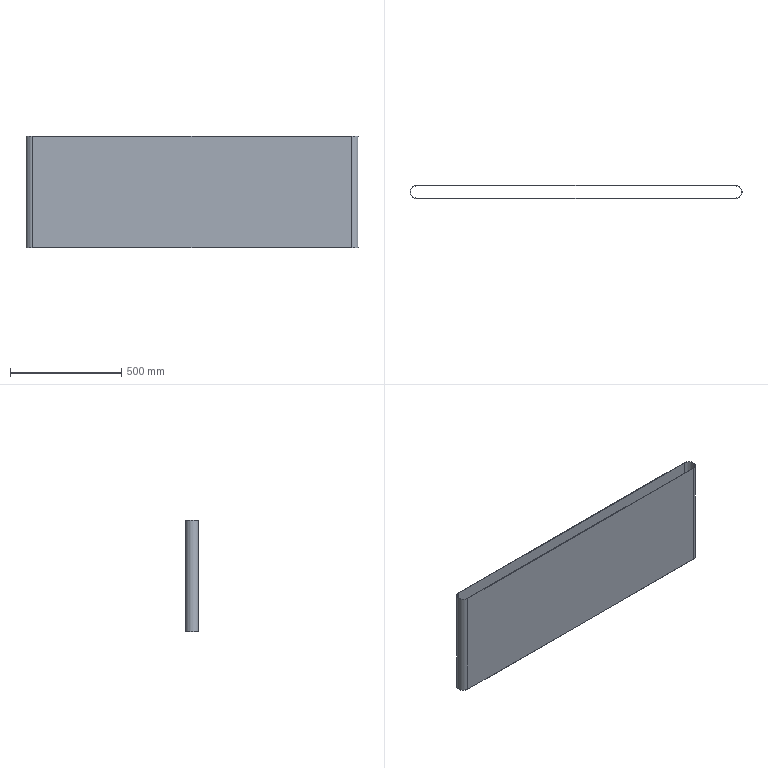Part | STEP file | RUBE Q7C | 1 solid | 10 faces | box 1492 x 59.6 x 500 mm | volume 2741026 mm3 | plane 6 | cylinder 4 | commonest cylinder face diameters 56 x2 59.6 x2
STEP:
#1=CARTESIAN_POINT('',(0.,0.,0.));
#2=DIRECTION('',(0.,0.,1.));
#3=DIRECTION('',(1.,0.,0.));
#4=AXIS2_PLACEMENT_3D('',#1,#2,#3);
#5=CARTESIAN_POINT('',(-1248.5,29.8,250.));
#6=VERTEX_POINT('',#5);
#7=CARTESIAN_POINT('',(-1248.5,-29.8,250.));
#8=VERTEX_POINT('',#7);
#9=CARTESIAN_POINT('',(-1248.5,0.,250.));
#10=DIRECTION('',(0.,0.,1.));
#11=DIRECTION('',(1.,0.,0.));
#12=AXIS2_PLACEMENT_3D('',#9,#10,#11);
#13=CIRCLE('',#12,29.8);
#14=CARTESIAN_POINT('',(-1248.5,0.,250.));
#15=DIRECTION('',(0.,0.,1.));
#16=DIRECTION('',(1.,0.,0.));
#17=AXIS2_PLACEMENT_3D('',#14,#15,#16);
#18=PLANE('',#17);
#19=CARTESIAN_POINT('',(0.,0.));
#20=DIRECTION('',(1.,0.));
#21=AXIS2_PLACEMENT_2D('',#19,#20);
#22=CIRCLE('',#21,29.8);
#23=(GEOMETRIC_REPRESENTATION_CONTEXT(2)PARAMETRIC_REPRESENTATION_CONTEXT()REPRESENTATION_CONTEXT('',''));
#24=DEFINITIONAL_REPRESENTATION('',(#22),#23);
#25=PCURVE('',#18,#24);
#26=CARTESIAN_POINT('',(-1248.5,0.,250.));
#27=DIRECTION('',(0.,0.,-1.));
#28=DIRECTION('',(-1.,0.,0.));
#29=AXIS2_PLACEMENT_3D('',#26,#27,#28);
#30=CYLINDRICAL_SURFACE('',#29,29.8);
#31=CARTESIAN_POINT('',(3.142,0.));
#32=DIRECTION('',(-1.,0.));
#33=VECTOR('',#32,1.);
#34=LINE('',#31,#33);
#35=(GEOMETRIC_REPRESENTATION_CONTEXT(2)PARAMETRIC_REPRESENTATION_CONTEXT()REPRESENTATION_CONTEXT('',''));
#36=DEFINITIONAL_REPRESENTATION('',(#34),#35);
#37=PCURVE('',#30,#36);
#38=SURFACE_CURVE('',#13,(#25,#37),.PCURVE_S1.);
#39=EDGE_CURVE('',#6,#8,#38,.T.);
#40=ORIENTED_EDGE('',*,*,#39,.T.);
#41=CARTESIAN_POINT('',(183.5,-29.8,250.));
#42=VERTEX_POINT('',#41);
#43=CARTESIAN_POINT('',(-1248.5,-29.8,250.));
#44=DIRECTION('',(1.,0.,0.));
#45=VECTOR('',#44,1.);
#46=LINE('',#43,#45);
#47=CARTESIAN_POINT('',(0.,-29.8));
#48=DIRECTION('',(1.,0.));
#49=VECTOR('',#48,1.);
#50=LINE('',#47,#49);
#51=(GEOMETRIC_REPRESENTATION_CONTEXT(2)PARAMETRIC_REPRESENTATION_CONTEXT()REPRESENTATION_CONTEXT('',''));
#52=DEFINITIONAL_REPRESENTATION('',(#50),#51);
#53=PCURVE('',#18,#52);
#54=CARTESIAN_POINT('',(-1248.5,-29.8,250.));
#55=DIRECTION('',(0.,1.,0.));
#56=DIRECTION('',(-1.,0.,0.));
#57=AXIS2_PLACEMENT_3D('',#54,#55,#56);
#58=PLANE('',#57);
#59=CARTESIAN_POINT('',(0.,0.));
#60=DIRECTION('',(-1.,0.));
#61=VECTOR('',#60,1.);
#62=LINE('',#59,#61);
#63=(GEOMETRIC_REPRESENTATION_CONTEXT(2)PARAMETRIC_REPRESENTATION_CONTEXT()REPRESENTATION_CONTEXT('',''));
#64=DEFINITIONAL_REPRESENTATION('',(#62),#63);
#65=PCURVE('',#58,#64);
#66=SURFACE_CURVE('',#46,(#53,#65),.PCURVE_S1.);
#67=EDGE_CURVE('',#8,#42,#66,.T.);
#68=ORIENTED_EDGE('',*,*,#67,.T.);
#69=CARTESIAN_POINT('',(183.5,29.8,250.));
#70=VERTEX_POINT('',#69);
#71=CARTESIAN_POINT('',(183.5,0.,250.));
#72=DIRECTION('',(0.,0.,1.));
#73=DIRECTION('',(1.,0.,0.));
#74=AXIS2_PLACEMENT_3D('',#71,#72,#73);
#75=CIRCLE('',#74,29.8);
#76=CARTESIAN_POINT('',(1432.,0.));
#77=DIRECTION('',(1.,0.));
#78=AXIS2_PLACEMENT_2D('',#76,#77);
#79=CIRCLE('',#78,29.8);
#80=(GEOMETRIC_REPRESENTATION_CONTEXT(2)PARAMETRIC_REPRESENTATION_CONTEXT()REPRESENTATION_CONTEXT('',''));
#81=DEFINITIONAL_REPRESENTATION('',(#79),#80);
#82=PCURVE('',#18,#81);
#83=CARTESIAN_POINT('',(183.5,0.,250.));
#84=DIRECTION('',(0.,0.,-1.));
#85=DIRECTION('',(-1.,0.,0.));
#86=AXIS2_PLACEMENT_3D('',#83,#84,#85);
#87=CYLINDRICAL_SURFACE('',#86,29.8);
#88=CARTESIAN_POINT('',(9.425,0.));
#89=DIRECTION('',(-1.,0.));
#90=VECTOR('',#89,1.);
#91=LINE('',#88,#90);
#92=(GEOMETRIC_REPRESENTATION_CONTEXT(2)PARAMETRIC_REPRESENTATION_CONTEXT()REPRESENTATION_CONTEXT('',''));
#93=DEFINITIONAL_REPRESENTATION('',(#91),#92);
#94=PCURVE('',#87,#93);
#95=SURFACE_CURVE('',#75,(#82,#94),.PCURVE_S1.);
#96=EDGE_CURVE('',#42,#70,#95,.T.);
#97=ORIENTED_EDGE('',*,*,#96,.T.);
#98=CARTESIAN_POINT('',(-1248.5,29.8,250.));
#99=DIRECTION('',(-1.,0.,0.));
#100=VECTOR('',#99,1.);
#101=LINE('',#98,#100);
#102=CARTESIAN_POINT('',(0.,29.8));
#103=DIRECTION('',(-1.,0.));
#104=VECTOR('',#103,1.);
#105=LINE('',#102,#104);
#106=(GEOMETRIC_REPRESENTATION_CONTEXT(2)PARAMETRIC_REPRESENTATION_CONTEXT()REPRESENTATION_CONTEXT('',''));
#107=DEFINITIONAL_REPRESENTATION('',(#105),#106);
#108=PCURVE('',#18,#107);
#109=CARTESIAN_POINT('',(-1248.5,29.8,250.));
#110=DIRECTION('',(0.,-1.,0.));
#111=DIRECTION('',(1.,0.,0.));
#112=AXIS2_PLACEMENT_3D('',#109,#110,#111);
#113=PLANE('',#112);
#114=CARTESIAN_POINT('',(0.,0.));
#115=DIRECTION('',(-1.,0.));
#116=VECTOR('',#115,1.);
#117=LINE('',#114,#116);
#118=(GEOMETRIC_REPRESENTATION_CONTEXT(2)PARAMETRIC_REPRESENTATION_CONTEXT()REPRESENTATION_CONTEXT('',''));
#119=DEFINITIONAL_REPRESENTATION('',(#117),#118);
#120=PCURVE('',#113,#119);
#121=SURFACE_CURVE('',#101,(#108,#120),.PCURVE_S1.);
#122=EDGE_CURVE('',#70,#6,#121,.T.);
#123=ORIENTED_EDGE('',*,*,#122,.T.);
#124=EDGE_LOOP('',(#40,#68,#97,#123));
#125=FACE_BOUND('',#124,.T.);
#126=CARTESIAN_POINT('',(-1248.5,-28.,250.));
#127=VERTEX_POINT('',#126);
#128=CARTESIAN_POINT('',(183.5,-28.,250.));
#129=VERTEX_POINT('',#128);
#130=CARTESIAN_POINT('',(-1248.5,-28.,250.));
#131=DIRECTION('',(1.,0.,0.));
#132=VECTOR('',#131,1.);
#133=LINE('',#130,#132);
#134=CARTESIAN_POINT('',(0.,-28.));
#135=DIRECTION('',(1.,0.));
#136=VECTOR('',#135,1.);
#137=LINE('',#134,#136);
#138=(GEOMETRIC_REPRESENTATION_CONTEXT(2)PARAMETRIC_REPRESENTATION_CONTEXT()REPRESENTATION_CONTEXT('',''));
#139=DEFINITIONAL_REPRESENTATION('',(#137),#138);
#140=PCURVE('',#18,#139);
#141=CARTESIAN_POINT('',(-1248.5,-28.,250.));
#142=DIRECTION('',(0.,1.,0.));
#143=DIRECTION('',(-1.,0.,0.));
#144=AXIS2_PLACEMENT_3D('',#141,#142,#143);
#145=PLANE('',#144);
#146=CARTESIAN_POINT('',(0.,0.));
#147=DIRECTION('',(-1.,0.));
#148=VECTOR('',#147,1.);
#149=LINE('',#146,#148);
#150=(GEOMETRIC_REPRESENTATION_CONTEXT(2)PARAMETRIC_REPRESENTATION_CONTEXT()REPRESENTATION_CONTEXT('',''));
#151=DEFINITIONAL_REPRESENTATION('',(#149),#150);
#152=PCURVE('',#145,#151);
#153=SURFACE_CURVE('',#133,(#140,#152),.PCURVE_S1.);
#154=EDGE_CURVE('',#127,#129,#153,.T.);
#155=ORIENTED_EDGE('',*,*,#154,.F.);
#156=CARTESIAN_POINT('',(-1248.5,28.,250.));
#157=VERTEX_POINT('',#156);
#158=CARTESIAN_POINT('',(-1248.5,0.,250.));
#159=DIRECTION('',(0.,0.,1.));
#160=DIRECTION('',(1.,0.,0.));
#161=AXIS2_PLACEMENT_3D('',#158,#159,#160);
#162=CIRCLE('',#161,28.);
#163=CARTESIAN_POINT('',(0.,0.));
#164=DIRECTION('',(1.,0.));
#165=AXIS2_PLACEMENT_2D('',#163,#164);
#166=CIRCLE('',#165,28.);
#167=(GEOMETRIC_REPRESENTATION_CONTEXT(2)PARAMETRIC_REPRESENTATION_CONTEXT()REPRESENTATION_CONTEXT('',''));
#168=DEFINITIONAL_REPRESENTATION('',(#166),#167);
#169=PCURVE('',#18,#168);
#170=CARTESIAN_POINT('',(-1248.5,0.,250.));
#171=DIRECTION('',(0.,0.,-1.));
#172=DIRECTION('',(-1.,0.,0.));
#173=AXIS2_PLACEMENT_3D('',#170,#171,#172);
#174=CYLINDRICAL_SURFACE('',#173,28.);
#175=CARTESIAN_POINT('',(3.142,0.));
#176=DIRECTION('',(-1.,0.));
#177=VECTOR('',#176,1.);
#178=LINE('',#175,#177);
#179=(GEOMETRIC_REPRESENTATION_CONTEXT(2)PARAMETRIC_REPRESENTATION_CONTEXT()REPRESENTATION_CONTEXT('',''));
#180=DEFINITIONAL_REPRESENTATION('',(#178),#179);
#181=PCURVE('',#174,#180);
#182=SURFACE_CURVE('',#162,(#169,#181),.PCURVE_S1.);
#183=EDGE_CURVE('',#157,#127,#182,.T.);
#184=ORIENTED_EDGE('',*,*,#183,.F.);
#185=CARTESIAN_POINT('',(183.5,28.,250.));
#186=VERTEX_POINT('',#185);
#187=CARTESIAN_POINT('',(-1248.5,28.,250.));
#188=DIRECTION('',(-1.,0.,0.));
#189=VECTOR('',#188,1.);
#190=LINE('',#187,#189);
#191=CARTESIAN_POINT('',(0.,28.));
#192=DIRECTION('',(-1.,0.));
#193=VECTOR('',#192,1.);
#194=LINE('',#191,#193);
#195=(GEOMETRIC_REPRESENTATION_CONTEXT(2)PARAMETRIC_REPRESENTATION_CONTEXT()REPRESENTATION_CONTEXT('',''));
#196=DEFINITIONAL_REPRESENTATION('',(#194),#195);
#197=PCURVE('',#18,#196);
#198=CARTESIAN_POINT('',(-1248.5,28.,250.));
#199=DIRECTION('',(0.,-1.,0.));
#200=DIRECTION('',(1.,0.,0.));
#201=AXIS2_PLACEMENT_3D('',#198,#199,#200);
#202=PLANE('',#201);
#203=CARTESIAN_POINT('',(0.,0.));
#204=DIRECTION('',(-1.,0.));
#205=VECTOR('',#204,1.);
#206=LINE('',#203,#205);
#207=(GEOMETRIC_REPRESENTATION_CONTEXT(2)PARAMETRIC_REPRESENTATION_CONTEXT()REPRESENTATION_CONTEXT('',''));
#208=DEFINITIONAL_REPRESENTATION('',(#206),#207);
#209=PCURVE('',#202,#208);
#210=SURFACE_CURVE('',#190,(#197,#209),.PCURVE_S1.);
#211=EDGE_CURVE('',#186,#157,#210,.T.);
#212=ORIENTED_EDGE('',*,*,#211,.F.);
#213=CARTESIAN_POINT('',(183.5,0.,250.));
#214=DIRECTION('',(0.,0.,1.));
#215=DIRECTION('',(1.,0.,0.));
#216=AXIS2_PLACEMENT_3D('',#213,#214,#215);
#217=CIRCLE('',#216,28.);
#218=CARTESIAN_POINT('',(1432.,0.));
#219=DIRECTION('',(1.,0.));
#220=AXIS2_PLACEMENT_2D('',#218,#219);
#221=CIRCLE('',#220,28.);
#222=(GEOMETRIC_REPRESENTATION_CONTEXT(2)PARAMETRIC_REPRESENTATION_CONTEXT()REPRESENTATION_CONTEXT('',''));
#223=DEFINITIONAL_REPRESENTATION('',(#221),#222);
#224=PCURVE('',#18,#223);
#225=CARTESIAN_POINT('',(183.5,0.,250.));
#226=DIRECTION('',(0.,0.,-1.));
#227=DIRECTION('',(-1.,0.,0.));
#228=AXIS2_PLACEMENT_3D('',#225,#226,#227);
#229=CYLINDRICAL_SURFACE('',#228,28.);
#230=CARTESIAN_POINT('',(9.425,0.));
#231=DIRECTION('',(-1.,0.));
#232=VECTOR('',#231,1.);
#233=LINE('',#230,#232);
#234=(GEOMETRIC_REPRESENTATION_CONTEXT(2)PARAMETRIC_REPRESENTATION_CONTEXT()REPRESENTATION_CONTEXT('',''));
#235=DEFINITIONAL_REPRESENTATION('',(#233),#234);
#236=PCURVE('',#229,#235);
#237=SURFACE_CURVE('',#217,(#224,#236),.PCURVE_S1.);
#238=EDGE_CURVE('',#129,#186,#237,.T.);
#239=ORIENTED_EDGE('',*,*,#238,.F.);
#240=EDGE_LOOP('',(#155,#184,#212,#239));
#241=FACE_BOUND('',#240,.T.);
#242=ADVANCED_FACE('',(#125,#241),#18,.T.);
#243=CARTESIAN_POINT('',(-1248.5,29.8,-250.));
#244=VERTEX_POINT('',#243);
#245=CARTESIAN_POINT('',(-1248.5,-29.8,-250.));
#246=VERTEX_POINT('',#245);
#247=CARTESIAN_POINT('',(-1248.5,0.,-250.));
#248=DIRECTION('',(0.,0.,1.));
#249=DIRECTION('',(1.,0.,0.));
#250=AXIS2_PLACEMENT_3D('',#247,#248,#249);
#251=CIRCLE('',#250,29.8);
#252=CARTESIAN_POINT('',(-1248.5,0.,-250.));
#253=DIRECTION('',(0.,0.,1.));
#254=DIRECTION('',(1.,0.,0.));
#255=AXIS2_PLACEMENT_3D('',#252,#253,#254);
#256=PLANE('',#255);
#257=CARTESIAN_POINT('',(0.,0.));
#258=DIRECTION('',(1.,0.));
#259=AXIS2_PLACEMENT_2D('',#257,#258);
#260=CIRCLE('',#259,29.8);
#261=(GEOMETRIC_REPRESENTATION_CONTEXT(2)PARAMETRIC_REPRESENTATION_CONTEXT()REPRESENTATION_CONTEXT('',''));
#262=DEFINITIONAL_REPRESENTATION('',(#260),#261);
#263=PCURVE('',#256,#262);
#264=CARTESIAN_POINT('',(3.142,500.));
#265=DIRECTION('',(-1.,0.));
#266=VECTOR('',#265,1.);
#267=LINE('',#264,#266);
#268=(GEOMETRIC_REPRESENTATION_CONTEXT(2)PARAMETRIC_REPRESENTATION_CONTEXT()REPRESENTATION_CONTEXT('',''));
#269=DEFINITIONAL_REPRESENTATION('',(#267),#268);
#270=PCURVE('',#30,#269);
#271=SURFACE_CURVE('',#251,(#263,#270),.PCURVE_S1.);
#272=EDGE_CURVE('',#244,#246,#271,.T.);
#273=ORIENTED_EDGE('',*,*,#272,.F.);
#274=CARTESIAN_POINT('',(183.5,29.8,-250.));
#275=VERTEX_POINT('',#274);
#276=CARTESIAN_POINT('',(-1248.5,29.8,-250.));
#277=DIRECTION('',(-1.,0.,0.));
#278=VECTOR('',#277,1.);
#279=LINE('',#276,#278);
#280=CARTESIAN_POINT('',(0.,29.8));
#281=DIRECTION('',(-1.,0.));
#282=VECTOR('',#281,1.);
#283=LINE('',#280,#282);
#284=(GEOMETRIC_REPRESENTATION_CONTEXT(2)PARAMETRIC_REPRESENTATION_CONTEXT()REPRESENTATION_CONTEXT('',''));
#285=DEFINITIONAL_REPRESENTATION('',(#283),#284);
#286=PCURVE('',#256,#285);
#287=CARTESIAN_POINT('',(0.,-500.));
#288=DIRECTION('',(-1.,0.));
#289=VECTOR('',#288,1.);
#290=LINE('',#287,#289);
#291=(GEOMETRIC_REPRESENTATION_CONTEXT(2)PARAMETRIC_REPRESENTATION_CONTEXT()REPRESENTATION_CONTEXT('',''));
#292=DEFINITIONAL_REPRESENTATION('',(#290),#291);
#293=PCURVE('',#113,#292);
#294=SURFACE_CURVE('',#279,(#286,#293),.PCURVE_S1.);
#295=EDGE_CURVE('',#275,#244,#294,.T.);
#296=ORIENTED_EDGE('',*,*,#295,.F.);
#297=CARTESIAN_POINT('',(183.5,-29.8,-250.));
#298=VERTEX_POINT('',#297);
#299=CARTESIAN_POINT('',(183.5,0.,-250.));
#300=DIRECTION('',(0.,0.,1.));
#301=DIRECTION('',(1.,0.,0.));
#302=AXIS2_PLACEMENT_3D('',#299,#300,#301);
#303=CIRCLE('',#302,29.8);
#304=CARTESIAN_POINT('',(1432.,0.));
#305=DIRECTION('',(1.,0.));
#306=AXIS2_PLACEMENT_2D('',#304,#305);
#307=CIRCLE('',#306,29.8);
#308=(GEOMETRIC_REPRESENTATION_CONTEXT(2)PARAMETRIC_REPRESENTATION_CONTEXT()REPRESENTATION_CONTEXT('',''));
#309=DEFINITIONAL_REPRESENTATION('',(#307),#308);
#310=PCURVE('',#256,#309);
#311=CARTESIAN_POINT('',(9.425,500.));
#312=DIRECTION('',(-1.,0.));
#313=VECTOR('',#312,1.);
#314=LINE('',#311,#313);
#315=(GEOMETRIC_REPRESENTATION_CONTEXT(2)PARAMETRIC_REPRESENTATION_CONTEXT()REPRESENTATION_CONTEXT('',''));
#316=DEFINITIONAL_REPRESENTATION('',(#314),#315);
#317=PCURVE('',#87,#316);
#318=SURFACE_CURVE('',#303,(#310,#317),.PCURVE_S1.);
#319=EDGE_CURVE('',#298,#275,#318,.T.);
#320=ORIENTED_EDGE('',*,*,#319,.F.);
#321=CARTESIAN_POINT('',(-1248.5,-29.8,-250.));
#322=DIRECTION('',(1.,0.,0.));
#323=VECTOR('',#322,1.);
#324=LINE('',#321,#323);
#325=CARTESIAN_POINT('',(0.,-29.8));
#326=DIRECTION('',(1.,0.));
#327=VECTOR('',#326,1.);
#328=LINE('',#325,#327);
#329=(GEOMETRIC_REPRESENTATION_CONTEXT(2)PARAMETRIC_REPRESENTATION_CONTEXT()REPRESENTATION_CONTEXT('',''));
#330=DEFINITIONAL_REPRESENTATION('',(#328),#329);
#331=PCURVE('',#256,#330);
#332=CARTESIAN_POINT('',(0.,-500.));
#333=DIRECTION('',(-1.,0.));
#334=VECTOR('',#333,1.);
#335=LINE('',#332,#334);
#336=(GEOMETRIC_REPRESENTATION_CONTEXT(2)PARAMETRIC_REPRESENTATION_CONTEXT()REPRESENTATION_CONTEXT('',''));
#337=DEFINITIONAL_REPRESENTATION('',(#335),#336);
#338=PCURVE('',#58,#337);
#339=SURFACE_CURVE('',#324,(#331,#338),.PCURVE_S1.);
#340=EDGE_CURVE('',#246,#298,#339,.T.);
#341=ORIENTED_EDGE('',*,*,#340,.F.);
#342=EDGE_LOOP('',(#273,#296,#320,#341));
#343=FACE_BOUND('',#342,.T.);
#344=CARTESIAN_POINT('',(-1248.5,28.,-250.));
#345=VERTEX_POINT('',#344);
#346=CARTESIAN_POINT('',(-1248.5,-28.,-250.));
#347=VERTEX_POINT('',#346);
#348=CARTESIAN_POINT('',(-1248.5,0.,-250.));
#349=DIRECTION('',(0.,0.,1.));
#350=DIRECTION('',(1.,0.,0.));
#351=AXIS2_PLACEMENT_3D('',#348,#349,#350);
#352=CIRCLE('',#351,28.);
#353=CARTESIAN_POINT('',(0.,0.));
#354=DIRECTION('',(1.,0.));
#355=AXIS2_PLACEMENT_2D('',#353,#354);
#356=CIRCLE('',#355,28.);
#357=(GEOMETRIC_REPRESENTATION_CONTEXT(2)PARAMETRIC_REPRESENTATION_CONTEXT()REPRESENTATION_CONTEXT('',''));
#358=DEFINITIONAL_REPRESENTATION('',(#356),#357);
#359=PCURVE('',#256,#358);
#360=CARTESIAN_POINT('',(3.142,500.));
#361=DIRECTION('',(-1.,0.));
#362=VECTOR('',#361,1.);
#363=LINE('',#360,#362);
#364=(GEOMETRIC_REPRESENTATION_CONTEXT(2)PARAMETRIC_REPRESENTATION_CONTEXT()REPRESENTATION_CONTEXT('',''));
#365=DEFINITIONAL_REPRESENTATION('',(#363),#364);
#366=PCURVE('',#174,#365);
#367=SURFACE_CURVE('',#352,(#359,#366),.PCURVE_S1.);
#368=EDGE_CURVE('',#345,#347,#367,.T.);
#369=ORIENTED_EDGE('',*,*,#368,.T.);
#370=CARTESIAN_POINT('',(183.5,-28.,-250.));
#371=VERTEX_POINT('',#370);
#372=CARTESIAN_POINT('',(-1248.5,-28.,-250.));
#373=DIRECTION('',(1.,0.,0.));
#374=VECTOR('',#373,1.);
#375=LINE('',#372,#374);
#376=CARTESIAN_POINT('',(0.,-28.));
#377=DIRECTION('',(1.,0.));
#378=VECTOR('',#377,1.);
#379=LINE('',#376,#378);
#380=(GEOMETRIC_REPRESENTATION_CONTEXT(2)PARAMETRIC_REPRESENTATION_CONTEXT()REPRESENTATION_CONTEXT('',''));
#381=DEFINITIONAL_REPRESENTATION('',(#379),#380);
#382=PCURVE('',#256,#381);
#383=CARTESIAN_POINT('',(0.,-500.));
#384=DIRECTION('',(-1.,0.));
#385=VECTOR('',#384,1.);
#386=LINE('',#383,#385);
#387=(GEOMETRIC_REPRESENTATION_CONTEXT(2)PARAMETRIC_REPRESENTATION_CONTEXT()REPRESENTATION_CONTEXT('',''));
#388=DEFINITIONAL_REPRESENTATION('',(#386),#387);
#389=PCURVE('',#145,#388);
#390=SURFACE_CURVE('',#375,(#382,#389),.PCURVE_S1.);
#391=EDGE_CURVE('',#347,#371,#390,.T.);
#392=ORIENTED_EDGE('',*,*,#391,.T.);
#393=CARTESIAN_POINT('',(183.5,28.,-250.));
#394=VERTEX_POINT('',#393);
#395=CARTESIAN_POINT('',(183.5,0.,-250.));
#396=DIRECTION('',(0.,0.,1.));
#397=DIRECTION('',(1.,0.,0.));
#398=AXIS2_PLACEMENT_3D('',#395,#396,#397);
#399=CIRCLE('',#398,28.);
#400=CARTESIAN_POINT('',(1432.,0.));
#401=DIRECTION('',(1.,0.));
#402=AXIS2_PLACEMENT_2D('',#400,#401);
#403=CIRCLE('',#402,28.);
#404=(GEOMETRIC_REPRESENTATION_CONTEXT(2)PARAMETRIC_REPRESENTATION_CONTEXT()REPRESENTATION_CONTEXT('',''));
#405=DEFINITIONAL_REPRESENTATION('',(#403),#404);
#406=PCURVE('',#256,#405);
#407=CARTESIAN_POINT('',(9.425,500.));
#408=DIRECTION('',(-1.,0.));
#409=VECTOR('',#408,1.);
#410=LINE('',#407,#409);
#411=(GEOMETRIC_REPRESENTATION_CONTEXT(2)PARAMETRIC_REPRESENTATION_CONTEXT()REPRESENTATION_CONTEXT('',''));
#412=DEFINITIONAL_REPRESENTATION('',(#410),#411);
#413=PCURVE('',#229,#412);
#414=SURFACE_CURVE('',#399,(#406,#413),.PCURVE_S1.);
#415=EDGE_CURVE('',#371,#394,#414,.T.);
#416=ORIENTED_EDGE('',*,*,#415,.T.);
#417=CARTESIAN_POINT('',(-1248.5,28.,-250.));
#418=DIRECTION('',(-1.,0.,0.));
#419=VECTOR('',#418,1.);
#420=LINE('',#417,#419);
#421=CARTESIAN_POINT('',(0.,28.));
#422=DIRECTION('',(-1.,0.));
#423=VECTOR('',#422,1.);
#424=LINE('',#421,#423);
#425=(GEOMETRIC_REPRESENTATION_CONTEXT(2)PARAMETRIC_REPRESENTATION_CONTEXT()REPRESENTATION_CONTEXT('',''));
#426=DEFINITIONAL_REPRESENTATION('',(#424),#425);
#427=PCURVE('',#256,#426);
#428=CARTESIAN_POINT('',(0.,-500.));
#429=DIRECTION('',(-1.,0.));
#430=VECTOR('',#429,1.);
#431=LINE('',#428,#430);
#432=(GEOMETRIC_REPRESENTATION_CONTEXT(2)PARAMETRIC_REPRESENTATION_CONTEXT()REPRESENTATION_CONTEXT('',''));
#433=DEFINITIONAL_REPRESENTATION('',(#431),#432);
#434=PCURVE('',#202,#433);
#435=SURFACE_CURVE('',#420,(#427,#434),.PCURVE_S1.);
#436=EDGE_CURVE('',#394,#345,#435,.T.);
#437=ORIENTED_EDGE('',*,*,#436,.T.);
#438=EDGE_LOOP('',(#369,#392,#416,#437));
#439=FACE_BOUND('',#438,.T.);
#440=ADVANCED_FACE('',(#343,#439),#256,.F.);
#441=ORIENTED_EDGE('',*,*,#272,.T.);
#442=CARTESIAN_POINT('',(-1248.5,-29.8,250.));
#443=DIRECTION('',(0.,0.,-1.));
#444=VECTOR('',#443,1.);
#445=LINE('',#442,#444);
#446=CARTESIAN_POINT('',(-1.571,0.));
#447=DIRECTION('',(0.,1.));
#448=VECTOR('',#447,1.);
#449=LINE('',#446,#448);
#450=(GEOMETRIC_REPRESENTATION_CONTEXT(2)PARAMETRIC_REPRESENTATION_CONTEXT()REPRESENTATION_CONTEXT('',''));
#451=DEFINITIONAL_REPRESENTATION('',(#449),#450);
#452=PCURVE('',#30,#451);
#453=CARTESIAN_POINT('',(0.,0.));
#454=DIRECTION('',(0.,-1.));
#455=VECTOR('',#454,1.);
#456=LINE('',#453,#455);
#457=(GEOMETRIC_REPRESENTATION_CONTEXT(2)PARAMETRIC_REPRESENTATION_CONTEXT()REPRESENTATION_CONTEXT('',''));
#458=DEFINITIONAL_REPRESENTATION('',(#456),#457);
#459=PCURVE('',#58,#458);
#460=SURFACE_CURVE('',#445,(#452,#459),.PCURVE_S1.);
#461=EDGE_CURVE('',#8,#246,#460,.T.);
#462=ORIENTED_EDGE('',*,*,#461,.F.);
#463=ORIENTED_EDGE('',*,*,#39,.F.);
#464=CARTESIAN_POINT('',(-1248.5,29.8,250.));
#465=DIRECTION('',(0.,0.,-1.));
#466=VECTOR('',#465,1.);
#467=LINE('',#464,#466);
#468=CARTESIAN_POINT('',(1.571,0.));
#469=DIRECTION('',(0.,1.));
#470=VECTOR('',#469,1.);
#471=LINE('',#468,#470);
#472=(GEOMETRIC_REPRESENTATION_CONTEXT(2)PARAMETRIC_REPRESENTATION_CONTEXT()REPRESENTATION_CONTEXT('',''));
#473=DEFINITIONAL_REPRESENTATION('',(#471),#472);
#474=PCURVE('',#30,#473);
#475=CARTESIAN_POINT('',(0.,0.));
#476=DIRECTION('',(0.,-1.));
#477=VECTOR('',#476,1.);
#478=LINE('',#475,#477);
#479=(GEOMETRIC_REPRESENTATION_CONTEXT(2)PARAMETRIC_REPRESENTATION_CONTEXT()REPRESENTATION_CONTEXT('',''));
#480=DEFINITIONAL_REPRESENTATION('',(#478),#479);
#481=PCURVE('',#113,#480);
#482=SURFACE_CURVE('',#467,(#474,#481),.PCURVE_S1.);
#483=EDGE_CURVE('',#6,#244,#482,.T.);
#484=ORIENTED_EDGE('',*,*,#483,.T.);
#485=EDGE_LOOP('',(#441,#462,#463,#484));
#486=FACE_BOUND('',#485,.T.);
#487=ADVANCED_FACE('',(#486),#30,.T.);
#488=ORIENTED_EDGE('',*,*,#340,.T.);
#489=CARTESIAN_POINT('',(183.5,-29.8,250.));
#490=DIRECTION('',(0.,0.,-1.));
#491=VECTOR('',#490,1.);
#492=LINE('',#489,#491);
#493=CARTESIAN_POINT('',(-1432.,0.));
#494=DIRECTION('',(0.,-1.));
#495=VECTOR('',#494,1.);
#496=LINE('',#493,#495);
#497=(GEOMETRIC_REPRESENTATION_CONTEXT(2)PARAMETRIC_REPRESENTATION_CONTEXT()REPRESENTATION_CONTEXT('',''));
#498=DEFINITIONAL_REPRESENTATION('',(#496),#497);
#499=PCURVE('',#58,#498);
#500=CARTESIAN_POINT('',(4.712,0.));
#501=DIRECTION('',(0.,1.));
#502=VECTOR('',#501,1.);
#503=LINE('',#500,#502);
#504=(GEOMETRIC_REPRESENTATION_CONTEXT(2)PARAMETRIC_REPRESENTATION_CONTEXT()REPRESENTATION_CONTEXT('',''));
#505=DEFINITIONAL_REPRESENTATION('',(#503),#504);
#506=PCURVE('',#87,#505);
#507=SURFACE_CURVE('',#492,(#499,#506),.PCURVE_S1.);
#508=EDGE_CURVE('',#42,#298,#507,.T.);
#509=ORIENTED_EDGE('',*,*,#508,.F.);
#510=ORIENTED_EDGE('',*,*,#67,.F.);
#511=ORIENTED_EDGE('',*,*,#461,.T.);
#512=EDGE_LOOP('',(#488,#509,#510,#511));
#513=FACE_BOUND('',#512,.T.);
#514=ADVANCED_FACE('',(#513),#58,.F.);
#515=ORIENTED_EDGE('',*,*,#319,.T.);
#516=CARTESIAN_POINT('',(183.5,29.8,250.));
#517=DIRECTION('',(0.,0.,-1.));
#518=VECTOR('',#517,1.);
#519=LINE('',#516,#518);
#520=CARTESIAN_POINT('',(1.571,0.));
#521=DIRECTION('',(0.,1.));
#522=VECTOR('',#521,1.);
#523=LINE('',#520,#522);
#524=(GEOMETRIC_REPRESENTATION_CONTEXT(2)PARAMETRIC_REPRESENTATION_CONTEXT()REPRESENTATION_CONTEXT('',''));
#525=DEFINITIONAL_REPRESENTATION('',(#523),#524);
#526=PCURVE('',#87,#525);
#527=CARTESIAN_POINT('',(1432.,0.));
#528=DIRECTION('',(0.,-1.));
#529=VECTOR('',#528,1.);
#530=LINE('',#527,#529);
#531=(GEOMETRIC_REPRESENTATION_CONTEXT(2)PARAMETRIC_REPRESENTATION_CONTEXT()REPRESENTATION_CONTEXT('',''));
#532=DEFINITIONAL_REPRESENTATION('',(#530),#531);
#533=PCURVE('',#113,#532);
#534=SURFACE_CURVE('',#519,(#526,#533),.PCURVE_S1.);
#535=EDGE_CURVE('',#70,#275,#534,.T.);
#536=ORIENTED_EDGE('',*,*,#535,.F.);
#537=ORIENTED_EDGE('',*,*,#96,.F.);
#538=ORIENTED_EDGE('',*,*,#508,.T.);
#539=EDGE_LOOP('',(#515,#536,#537,#538));
#540=FACE_BOUND('',#539,.T.);
#541=ADVANCED_FACE('',(#540),#87,.T.);
#542=ORIENTED_EDGE('',*,*,#295,.T.);
#543=ORIENTED_EDGE('',*,*,#483,.F.);
#544=ORIENTED_EDGE('',*,*,#122,.F.);
#545=ORIENTED_EDGE('',*,*,#535,.T.);
#546=EDGE_LOOP('',(#542,#543,#544,#545));
#547=FACE_BOUND('',#546,.T.);
#548=ADVANCED_FACE('',(#547),#113,.F.);
#549=CARTESIAN_POINT('',(-1248.5,-28.,250.));
#550=DIRECTION('',(0.,0.,-1.));
#551=VECTOR('',#550,1.);
#552=LINE('',#549,#551);
#553=CARTESIAN_POINT('',(-1.571,0.));
#554=DIRECTION('',(0.,1.));
#555=VECTOR('',#554,1.);
#556=LINE('',#553,#555);
#557=(GEOMETRIC_REPRESENTATION_CONTEXT(2)PARAMETRIC_REPRESENTATION_CONTEXT()REPRESENTATION_CONTEXT('',''));
#558=DEFINITIONAL_REPRESENTATION('',(#556),#557);
#559=PCURVE('',#174,#558);
#560=CARTESIAN_POINT('',(0.,0.));
#561=DIRECTION('',(0.,-1.));
#562=VECTOR('',#561,1.);
#563=LINE('',#560,#562);
#564=(GEOMETRIC_REPRESENTATION_CONTEXT(2)PARAMETRIC_REPRESENTATION_CONTEXT()REPRESENTATION_CONTEXT('',''));
#565=DEFINITIONAL_REPRESENTATION('',(#563),#564);
#566=PCURVE('',#145,#565);
#567=SURFACE_CURVE('',#552,(#559,#566),.PCURVE_S1.);
#568=EDGE_CURVE('',#127,#347,#567,.T.);
#569=ORIENTED_EDGE('',*,*,#568,.F.);
#570=ORIENTED_EDGE('',*,*,#183,.F.);
#571=CARTESIAN_POINT('',(-1248.5,28.,250.));
#572=DIRECTION('',(0.,0.,-1.));
#573=VECTOR('',#572,1.);
#574=LINE('',#571,#573);
#575=CARTESIAN_POINT('',(1.571,0.));
#576=DIRECTION('',(0.,1.));
#577=VECTOR('',#576,1.);
#578=LINE('',#575,#577);
#579=(GEOMETRIC_REPRESENTATION_CONTEXT(2)PARAMETRIC_REPRESENTATION_CONTEXT()REPRESENTATION_CONTEXT('',''));
#580=DEFINITIONAL_REPRESENTATION('',(#578),#579);
#581=PCURVE('',#174,#580);
#582=CARTESIAN_POINT('',(0.,0.));
#583=DIRECTION('',(0.,-1.));
#584=VECTOR('',#583,1.);
#585=LINE('',#582,#584);
#586=(GEOMETRIC_REPRESENTATION_CONTEXT(2)PARAMETRIC_REPRESENTATION_CONTEXT()REPRESENTATION_CONTEXT('',''));
#587=DEFINITIONAL_REPRESENTATION('',(#585),#586);
#588=PCURVE('',#202,#587);
#589=SURFACE_CURVE('',#574,(#581,#588),.PCURVE_S1.);
#590=EDGE_CURVE('',#157,#345,#589,.T.);
#591=ORIENTED_EDGE('',*,*,#590,.T.);
#592=ORIENTED_EDGE('',*,*,#368,.T.);
#593=EDGE_LOOP('',(#569,#570,#591,#592));
#594=FACE_BOUND('',#593,.F.);
#595=ADVANCED_FACE('',(#594),#174,.F.);
#596=ORIENTED_EDGE('',*,*,#391,.F.);
#597=ORIENTED_EDGE('',*,*,#568,.F.);
#598=ORIENTED_EDGE('',*,*,#154,.T.);
#599=CARTESIAN_POINT('',(183.5,-28.,250.));
#600=DIRECTION('',(0.,0.,-1.));
#601=VECTOR('',#600,1.);
#602=LINE('',#599,#601);
#603=CARTESIAN_POINT('',(-1432.,0.));
#604=DIRECTION('',(0.,-1.));
#605=VECTOR('',#604,1.);
#606=LINE('',#603,#605);
#607=(GEOMETRIC_REPRESENTATION_CONTEXT(2)PARAMETRIC_REPRESENTATION_CONTEXT()REPRESENTATION_CONTEXT('',''));
#608=DEFINITIONAL_REPRESENTATION('',(#606),#607);
#609=PCURVE('',#145,#608);
#610=CARTESIAN_POINT('',(4.712,0.));
#611=DIRECTION('',(0.,1.));
#612=VECTOR('',#611,1.);
#613=LINE('',#610,#612);
#614=(GEOMETRIC_REPRESENTATION_CONTEXT(2)PARAMETRIC_REPRESENTATION_CONTEXT()REPRESENTATION_CONTEXT('',''));
#615=DEFINITIONAL_REPRESENTATION('',(#613),#614);
#616=PCURVE('',#229,#615);
#617=SURFACE_CURVE('',#602,(#609,#616),.PCURVE_S1.);
#618=EDGE_CURVE('',#129,#371,#617,.T.);
#619=ORIENTED_EDGE('',*,*,#618,.T.);
#620=EDGE_LOOP('',(#596,#597,#598,#619));
#621=FACE_BOUND('',#620,.T.);
#622=ADVANCED_FACE('',(#621),#145,.T.);
#623=CARTESIAN_POINT('',(183.5,28.,250.));
#624=DIRECTION('',(0.,0.,-1.));
#625=VECTOR('',#624,1.);
#626=LINE('',#623,#625);
#627=CARTESIAN_POINT('',(1.571,0.));
#628=DIRECTION('',(0.,1.));
#629=VECTOR('',#628,1.);
#630=LINE('',#627,#629);
#631=(GEOMETRIC_REPRESENTATION_CONTEXT(2)PARAMETRIC_REPRESENTATION_CONTEXT()REPRESENTATION_CONTEXT('',''));
#632=DEFINITIONAL_REPRESENTATION('',(#630),#631);
#633=PCURVE('',#229,#632);
#634=CARTESIAN_POINT('',(1432.,0.));
#635=DIRECTION('',(0.,-1.));
#636=VECTOR('',#635,1.);
#637=LINE('',#634,#636);
#638=(GEOMETRIC_REPRESENTATION_CONTEXT(2)PARAMETRIC_REPRESENTATION_CONTEXT()REPRESENTATION_CONTEXT('',''));
#639=DEFINITIONAL_REPRESENTATION('',(#637),#638);
#640=PCURVE('',#202,#639);
#641=SURFACE_CURVE('',#626,(#633,#640),.PCURVE_S1.);
#642=EDGE_CURVE('',#186,#394,#641,.T.);
#643=ORIENTED_EDGE('',*,*,#642,.F.);
#644=ORIENTED_EDGE('',*,*,#238,.F.);
#645=ORIENTED_EDGE('',*,*,#618,.T.);
#646=ORIENTED_EDGE('',*,*,#415,.T.);
#647=EDGE_LOOP('',(#643,#644,#645,#646));
#648=FACE_BOUND('',#647,.F.);
#649=ADVANCED_FACE('',(#648),#229,.F.);
#650=ORIENTED_EDGE('',*,*,#436,.F.);
#651=ORIENTED_EDGE('',*,*,#642,.F.);
#652=ORIENTED_EDGE('',*,*,#211,.T.);
#653=ORIENTED_EDGE('',*,*,#590,.T.);
#654=EDGE_LOOP('',(#650,#651,#652,#653));
#655=FACE_BOUND('',#654,.T.);
#656=ADVANCED_FACE('',(#655),#202,.T.);
#657=CLOSED_SHELL('',(#242,#440,#487,#514,#541,#548,#595,#622,#649,#656));
#658=MANIFOLD_SOLID_BREP('',#657);
#659=(LENGTH_UNIT()NAMED_UNIT(*)SI_UNIT(.MILLI.,.METRE.));
#660=UNCERTAINTY_MEASURE_WITH_UNIT(LENGTH_MEASURE(0.0000001),#659,'','');
#661=(NAMED_UNIT(*)PLANE_ANGLE_UNIT()SI_UNIT($,.RADIAN.));
#662=(NAMED_UNIT(*)SI_UNIT($,.STERADIAN.)SOLID_ANGLE_UNIT());
#663=(GEOMETRIC_REPRESENTATION_CONTEXT(3)GLOBAL_UNCERTAINTY_ASSIGNED_CONTEXT((#660))GLOBAL_UNIT_ASSIGNED_CONTEXT((#659,#661,#662))REPRESENTATION_CONTEXT('',''));
#664=ADVANCED_BREP_SHAPE_REPRESENTATION('',(#4,#658),#663);